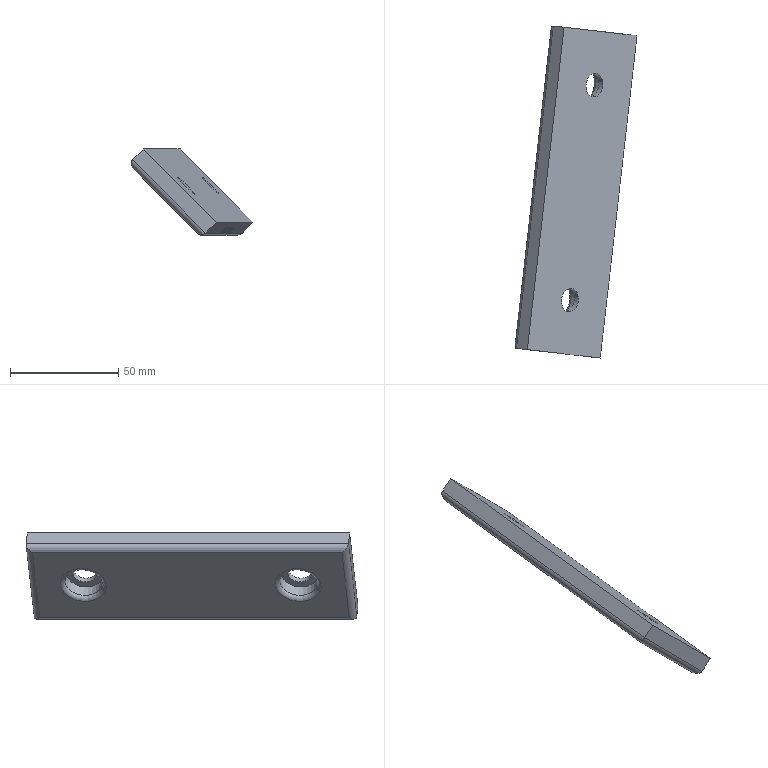Part | NX | features XQ 2 | 1 solid | 155 faces | box 56.404 x 153.447 x 39.77 mm | volume 67054 mm3 | plane 109 | spline 36 | cylinder 8 | torus 2 | commonest cylinder face diameters 6 x4 11 x2 17.5 x2